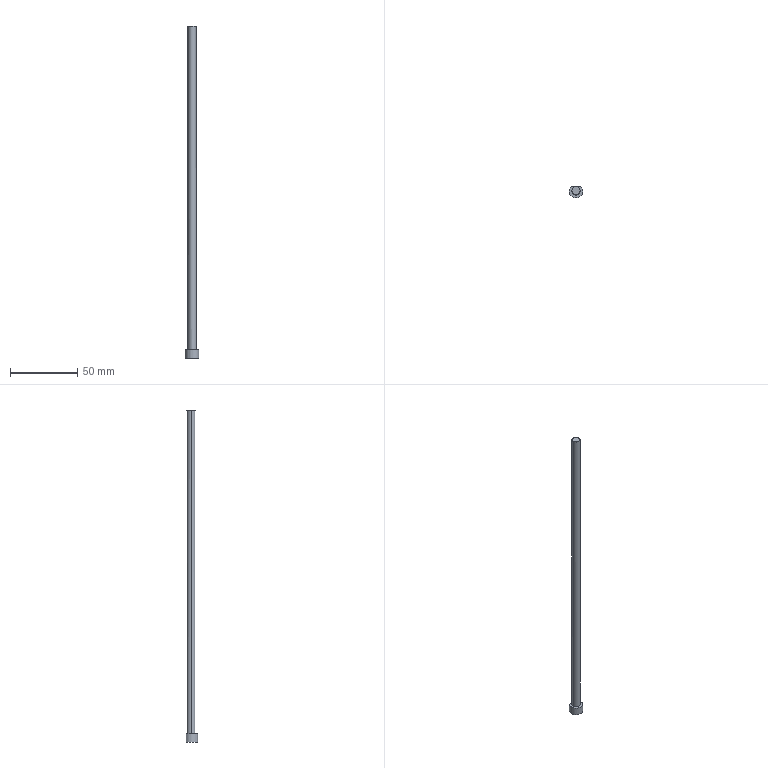Part | Creo | 1 solid | 7 faces | box 10 x 8.5 x 246.825 mm | volume 7236 mm3 | plane 4 | cylinder 3 | commonest cylinder face diameters 6 x2 10 x1
STEP:
#1=CARTESIAN_POINT('',(0.,0.,0.));
#2=DIRECTION('',(0.,0.,1.));
#3=DIRECTION('',(1.,0.,0.));
#4=AXIS2_PLACEMENT_3D('',#1,#2,#3);
#5=CARTESIAN_POINT('',(84.027,-19.769,-332.441));
#6=VERTEX_POINT('',#5);
#7=CARTESIAN_POINT('',(76.886,-19.769,-332.441));
#8=VERTEX_POINT('',#7);
#9=CARTESIAN_POINT('',(84.027,-19.769,-332.441));
#10=DIRECTION('',(-1.,0.,0.));
#11=VECTOR('',#10,7.141);
#12=LINE('',#9,#11);
#13=EDGE_CURVE('',#6,#8,#12,.T.);
#14=ORIENTED_EDGE('',*,*,#13,.F.);
#15=CARTESIAN_POINT('',(80.456,-23.269,-332.441));
#16=DIRECTION('',(0.,0.,-1.));
#17=DIRECTION('',(0.7141,0.7,0.));
#18=AXIS2_PLACEMENT_3D('',#15,#16,#17);
#19=CIRCLE('',#18,5.);
#20=EDGE_CURVE('',#6,#8,#19,.T.);
#21=ORIENTED_EDGE('',*,*,#20,.T.);
#22=EDGE_LOOP('',(#14,#21));
#23=FACE_OUTER_BOUND('',#22,.F.);
#24=CARTESIAN_POINT('',(77.456,-23.269,-332.441));
#25=VERTEX_POINT('',#24);
#26=CARTESIAN_POINT('',(83.456,-23.269,-332.441));
#27=VERTEX_POINT('',#26);
#28=CARTESIAN_POINT('',(80.456,-23.269,-332.441));
#29=DIRECTION('',(0.,0.,-1.));
#30=DIRECTION('',(-1.,0.,0.));
#31=AXIS2_PLACEMENT_3D('',#28,#29,#30);
#32=CIRCLE('',#31,3.);
#33=EDGE_CURVE('',#25,#27,#32,.T.);
#34=ORIENTED_EDGE('',*,*,#33,.F.);
#35=CARTESIAN_POINT('',(80.456,-23.269,-332.441));
#36=DIRECTION('',(0.,0.,-1.));
#37=DIRECTION('',(1.,0.,0.));
#38=AXIS2_PLACEMENT_3D('',#35,#36,#37);
#39=CIRCLE('',#38,3.);
#40=EDGE_CURVE('',#27,#25,#39,.T.);
#41=ORIENTED_EDGE('',*,*,#40,.F.);
#42=EDGE_LOOP('',(#34,#41));
#43=FACE_BOUND('',#42,.F.);
#44=CARTESIAN_POINT('',(80.456,-23.269,-332.441));
#45=DIRECTION('',(0.,0.,-1.));
#46=DIRECTION('',(-1.,0.,0.));
#47=AXIS2_PLACEMENT_3D('',#44,#45,#46);
#48=PLANE('',#47);
#49=ADVANCED_FACE('',(#23,#43),#48,.F.);
#50=CARTESIAN_POINT('',(83.456,-23.269,-91.624));
#51=VERTEX_POINT('',#50);
#52=CARTESIAN_POINT('',(77.456,-23.267,-91.617));
#53=VERTEX_POINT('',#52);
#54=CARTESIAN_POINT('',(83.456,-23.269,-91.624));
#55=CARTESIAN_POINT('',(83.456,-22.94,-91.624));
#56=CARTESIAN_POINT('',(83.354,-22.319,-91.624));
#57=CARTESIAN_POINT('',(82.915,-21.463,-91.624));
#58=CARTESIAN_POINT('',(82.238,-20.795,-91.623));
#59=CARTESIAN_POINT('',(81.392,-20.367,-91.622));
#60=CARTESIAN_POINT('',(80.458,-20.22,-91.621));
#61=CARTESIAN_POINT('',(79.524,-20.366,-91.619));
#62=CARTESIAN_POINT('',(78.677,-20.792,-91.618));
#63=CARTESIAN_POINT('',(78.,-21.46,-91.617));
#64=CARTESIAN_POINT('',(77.56,-22.314,-91.617));
#65=CARTESIAN_POINT('',(77.456,-22.938,-91.617));
#66=CARTESIAN_POINT('',(77.456,-23.267,-91.617));
#67=B_SPLINE_CURVE_WITH_KNOTS('',3,(#54,#55,#56,#57,#58,#59,#60,#61,#62,#63,#64,#65,#66),.UNSPECIFIED.,.F.,.F.,(4,1,1,1,1,1,1,1,1,1,4),(0.,0.1,0.2,0.3,0.4,0.5,0.6,0.7,0.8,0.9,1.),.UNSPECIFIED.);
#68=EDGE_CURVE('',#51,#53,#67,.T.);
#69=ORIENTED_EDGE('',*,*,#68,.T.);
#70=CARTESIAN_POINT('',(77.456,-23.269,-332.441));
#71=DIRECTION('',(0.000000003,0.000005269,1.));
#72=VECTOR('',#71,240.825);
#73=LINE('',#70,#72);
#74=EDGE_CURVE('',#25,#53,#73,.T.);
#75=ORIENTED_EDGE('',*,*,#74,.F.);
#76=ORIENTED_EDGE('',*,*,#33,.T.);
#77=CARTESIAN_POINT('',(83.456,-23.269,-332.441));
#78=DIRECTION('',(0.,0.,1.));
#79=VECTOR('',#78,240.817);
#80=LINE('',#77,#79);
#81=EDGE_CURVE('',#27,#51,#80,.T.);
#82=ORIENTED_EDGE('',*,*,#81,.T.);
#83=EDGE_LOOP('',(#69,#75,#76,#82));
#84=FACE_OUTER_BOUND('',#83,.F.);
#85=CARTESIAN_POINT('',(80.456,-23.269,-653.441));
#86=DIRECTION('',(0.,0.,1.));
#87=DIRECTION('',(1.,0.,0.));
#88=AXIS2_PLACEMENT_3D('',#85,#86,#87);
#89=CYLINDRICAL_SURFACE('',#88,3.);
#90=ADVANCED_FACE('',(#84),#89,.T.);
#91=CARTESIAN_POINT('',(77.456,-23.267,-91.617));
#92=CARTESIAN_POINT('',(77.456,-23.598,-91.617));
#93=CARTESIAN_POINT('',(77.558,-24.215,-91.617));
#94=CARTESIAN_POINT('',(77.997,-25.073,-91.617));
#95=CARTESIAN_POINT('',(78.663,-25.733,-91.618));
#96=CARTESIAN_POINT('',(79.502,-26.165,-91.619));
#97=CARTESIAN_POINT('',(80.444,-26.318,-91.621));
#98=CARTESIAN_POINT('',(81.386,-26.173,-91.622));
#99=CARTESIAN_POINT('',(82.231,-25.747,-91.623));
#100=CARTESIAN_POINT('',(82.908,-25.085,-91.624));
#101=CARTESIAN_POINT('',(83.354,-24.219,-91.624));
#102=CARTESIAN_POINT('',(83.456,-23.598,-91.624));
#103=CARTESIAN_POINT('',(83.456,-23.269,-91.624));
#104=B_SPLINE_CURVE_WITH_KNOTS('',3,(#91,#92,#93,#94,#95,#96,#97,#98,#99,#100,#101,#102,#103),.UNSPECIFIED.,.F.,.F.,(4,1,1,1,1,1,1,1,1,1,4),(0.,0.1,0.2,0.3,0.4,0.5,0.6,0.7,0.8,0.9,1.),.UNSPECIFIED.);
#105=EDGE_CURVE('',#53,#51,#104,.T.);
#106=ORIENTED_EDGE('',*,*,#105,.F.);
#107=ORIENTED_EDGE('',*,*,#68,.F.);
#108=EDGE_LOOP('',(#106,#107));
#109=FACE_OUTER_BOUND('',#108,.F.);
#110=CARTESIAN_POINT('',(248.993,54.022,-91.842));
#111=DIRECTION('',(-0.001312,0.000001665,-1.));
#112=DIRECTION('',(-1.,0.,0.001312));
#113=AXIS2_PLACEMENT_3D('',#110,#111,#112);
#114=PLANE('',#113);
#115=ADVANCED_FACE('',(#109),#114,.F.);
#116=ORIENTED_EDGE('',*,*,#105,.T.);
#117=ORIENTED_EDGE('',*,*,#81,.F.);
#118=ORIENTED_EDGE('',*,*,#40,.T.);
#119=ORIENTED_EDGE('',*,*,#74,.T.);
#120=EDGE_LOOP('',(#116,#117,#118,#119));
#121=FACE_OUTER_BOUND('',#120,.F.);
#122=CARTESIAN_POINT('',(80.456,-23.269,-653.441));
#123=DIRECTION('',(0.,0.,1.));
#124=DIRECTION('',(1.,0.,0.));
#125=AXIS2_PLACEMENT_3D('',#122,#123,#124);
#126=CYLINDRICAL_SURFACE('',#125,3.);
#127=ADVANCED_FACE('',(#121),#126,.T.);
#128=CARTESIAN_POINT('',(76.886,-19.769,-338.441));
#129=VERTEX_POINT('',#128);
#130=CARTESIAN_POINT('',(76.886,-19.769,-332.441));
#131=DIRECTION('',(0.,0.,-1.));
#132=VECTOR('',#131,6.);
#133=LINE('',#130,#132);
#134=EDGE_CURVE('',#8,#129,#133,.T.);
#135=ORIENTED_EDGE('',*,*,#134,.T.);
#136=CARTESIAN_POINT('',(84.027,-19.769,-338.441));
#137=VERTEX_POINT('',#136);
#138=CARTESIAN_POINT('',(84.027,-19.769,-338.441));
#139=DIRECTION('',(-1.,0.,0.));
#140=VECTOR('',#139,7.141);
#141=LINE('',#138,#140);
#142=EDGE_CURVE('',#137,#129,#141,.T.);
#143=ORIENTED_EDGE('',*,*,#142,.F.);
#144=CARTESIAN_POINT('',(84.027,-19.769,-338.441));
#145=DIRECTION('',(0.,0.,1.));
#146=VECTOR('',#145,6.);
#147=LINE('',#144,#146);
#148=EDGE_CURVE('',#137,#6,#147,.T.);
#149=ORIENTED_EDGE('',*,*,#148,.T.);
#150=ORIENTED_EDGE('',*,*,#13,.T.);
#151=EDGE_LOOP('',(#135,#143,#149,#150));
#152=FACE_OUTER_BOUND('',#151,.F.);
#153=CARTESIAN_POINT('',(80.456,-19.769,-338.441));
#154=DIRECTION('',(0.,1.,0.));
#155=DIRECTION('',(0.,0.,1.));
#156=AXIS2_PLACEMENT_3D('',#153,#154,#155);
#157=PLANE('',#156);
#158=ADVANCED_FACE('',(#152),#157,.T.);
#159=CARTESIAN_POINT('',(80.456,-23.269,-338.441));
#160=DIRECTION('',(0.,0.,1.));
#161=DIRECTION('',(-0.7141,0.7,0.));
#162=AXIS2_PLACEMENT_3D('',#159,#160,#161);
#163=CIRCLE('',#162,5.);
#164=EDGE_CURVE('',#129,#137,#163,.T.);
#165=ORIENTED_EDGE('',*,*,#164,.F.);
#166=ORIENTED_EDGE('',*,*,#134,.F.);
#167=ORIENTED_EDGE('',*,*,#20,.F.);
#168=ORIENTED_EDGE('',*,*,#148,.F.);
#169=EDGE_LOOP('',(#165,#166,#167,#168));
#170=FACE_OUTER_BOUND('',#169,.F.);
#171=CARTESIAN_POINT('',(80.456,-23.269,-332.441));
#172=DIRECTION('',(0.,0.,-1.));
#173=DIRECTION('',(-1.,0.,0.));
#174=AXIS2_PLACEMENT_3D('',#171,#172,#173);
#175=CYLINDRICAL_SURFACE('',#174,5.);
#176=ADVANCED_FACE('',(#170),#175,.T.);
#177=ORIENTED_EDGE('',*,*,#164,.T.);
#178=ORIENTED_EDGE('',*,*,#142,.T.);
#179=EDGE_LOOP('',(#177,#178));
#180=FACE_OUTER_BOUND('',#179,.F.);
#181=CARTESIAN_POINT('',(80.456,-23.269,-338.441));
#182=DIRECTION('',(0.,0.,-1.));
#183=DIRECTION('',(-1.,0.,0.));
#184=AXIS2_PLACEMENT_3D('',#181,#182,#183);
#185=PLANE('',#184);
#186=ADVANCED_FACE('',(#180),#185,.T.);
#187=CLOSED_SHELL('',(#49,#90,#115,#127,#158,#176,#186));
#188=MANIFOLD_SOLID_BREP('',#187);
#189=(LENGTH_UNIT()NAMED_UNIT(*)SI_UNIT(.MILLI.,.METRE.));
#190=UNCERTAINTY_MEASURE_WITH_UNIT(LENGTH_MEASURE(0.02472),#189,'','');
#191=(NAMED_UNIT(*)PLANE_ANGLE_UNIT()SI_UNIT($,.RADIAN.));
#192=PLANE_ANGLE_MEASURE_WITH_UNIT(PLANE_ANGLE_MEASURE(0.01745),#191);
#193=(CONVERSION_BASED_UNIT('DEGREE',#192)NAMED_UNIT(*)PLANE_ANGLE_UNIT());
#194=(NAMED_UNIT(*)SI_UNIT($,.STERADIAN.)SOLID_ANGLE_UNIT());
#195=(GEOMETRIC_REPRESENTATION_CONTEXT(3)GLOBAL_UNCERTAINTY_ASSIGNED_CONTEXT((#190))GLOBAL_UNIT_ASSIGNED_CONTEXT((#189,#193,#194))REPRESENTATION_CONTEXT('',''));
#196=ADVANCED_BREP_SHAPE_REPRESENTATION('',(#4,#188),#195);